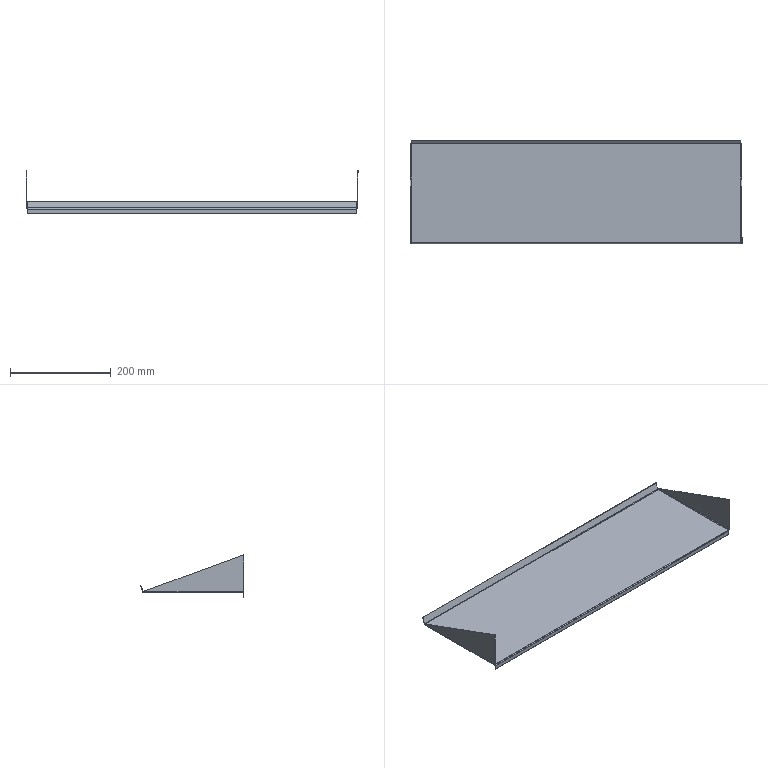Part | SolidWorks | features BaseBody 1 | 1 solid | 34 faces | box 660 x 205.13 x 84 mm | volume 161412 mm3 | plane 26 | cylinder 8 | commonest cylinder face diameters 2 x4 4 x4
STEP:
#1=CARTESIAN_POINT('',(-2.,2.,0.));
#2=VERTEX_POINT('',#1);
#3=CARTESIAN_POINT('',(-2.,198.6,0.));
#4=VERTEX_POINT('',#3);
#5=CARTESIAN_POINT('',(-2.,198.6,0.));
#6=DIRECTION('',(0.,1.,0.));
#7=VECTOR('',#6,1000.);
#8=LINE('',#5,#7);
#9=EDGE_CURVE('',#2,#4,#8,.T.);
#10=ORIENTED_EDGE('',*,*,#9,.F.);
#11=CARTESIAN_POINT('',(-658.,2.,0.));
#12=VERTEX_POINT('',#11);
#13=CARTESIAN_POINT('',(-660.262,2.,0.));
#14=DIRECTION('',(1.,0.,0.));
#15=VECTOR('',#14,1000.);
#16=LINE('',#13,#15);
#17=EDGE_CURVE('',#12,#2,#16,.T.);
#18=ORIENTED_EDGE('',*,*,#17,.F.);
#19=CARTESIAN_POINT('',(-658.,198.6,0.));
#20=VERTEX_POINT('',#19);
#21=CARTESIAN_POINT('',(-658.,198.6,0.));
#22=DIRECTION('',(0.,-1.,0.));
#23=VECTOR('',#22,1000.);
#24=LINE('',#21,#23);
#25=EDGE_CURVE('',#20,#12,#24,.T.);
#26=ORIENTED_EDGE('',*,*,#25,.F.);
#27=CARTESIAN_POINT('',(-660.262,198.6,0.));
#28=DIRECTION('',(-1.,0.,0.));
#29=VECTOR('',#28,1000.);
#30=LINE('',#27,#29);
#31=EDGE_CURVE('',#4,#20,#30,.T.);
#32=ORIENTED_EDGE('',*,*,#31,.F.);
#33=EDGE_LOOP('',(#10,#18,#26,#32));
#34=FACE_OUTER_BOUND('',#33,.T.);
#35=CARTESIAN_POINT('',(-660.262,198.6,0.));
#36=DIRECTION('',(0.,0.,1.));
#37=DIRECTION('',(1.,0.,0.));
#38=AXIS2_PLACEMENT_3D('',#35,#36,#37);
#39=PLANE('',#38);
#40=ADVANCED_FACE('',(#34),#39,.F.);
#41=CARTESIAN_POINT('',(-658.,200.479,1.316));
#42=VERTEX_POINT('',#41);
#43=CARTESIAN_POINT('',(-658.,198.6,2.));
#44=DIRECTION('',(1.,0.,0.));
#45=DIRECTION('',(0.,1.,0.));
#46=AXIS2_PLACEMENT_3D('',#43,#44,#45);
#47=CIRCLE('',#46,2.);
#48=EDGE_CURVE('',#20,#42,#47,.T.);
#49=ORIENTED_EDGE('',*,*,#48,.T.);
#50=CARTESIAN_POINT('',(-2.,200.479,1.316));
#51=VERTEX_POINT('',#50);
#52=CARTESIAN_POINT('',(-330.,200.479,1.316));
#53=DIRECTION('',(1.,0.,0.));
#54=VECTOR('',#53,1000.);
#55=LINE('',#52,#54);
#56=EDGE_CURVE('',#42,#51,#55,.T.);
#57=ORIENTED_EDGE('',*,*,#56,.T.);
#58=CARTESIAN_POINT('',(-2.,198.6,2.));
#59=DIRECTION('',(-1.,0.,0.));
#60=DIRECTION('',(0.,1.,0.));
#61=AXIS2_PLACEMENT_3D('',#58,#59,#60);
#62=CIRCLE('',#61,2.);
#63=EDGE_CURVE('',#51,#4,#62,.T.);
#64=ORIENTED_EDGE('',*,*,#63,.T.);
#65=ORIENTED_EDGE('',*,*,#31,.T.);
#66=EDGE_LOOP('',(#49,#57,#64,#65));
#67=FACE_OUTER_BOUND('',#66,.T.);
#68=CARTESIAN_POINT('',(-330.,198.6,2.));
#69=DIRECTION('',(1.,0.,0.));
#70=DIRECTION('',(0.,1.,0.));
#71=AXIS2_PLACEMENT_3D('',#68,#69,#70);
#72=CYLINDRICAL_SURFACE('',#71,2.);
#73=ADVANCED_FACE('',(#67),#72,.T.);
#74=CARTESIAN_POINT('',(0.,2.,2.));
#75=VERTEX_POINT('',#74);
#76=CARTESIAN_POINT('',(-2.,2.,2.));
#77=DIRECTION('',(0.,1.,0.));
#78=DIRECTION('',(1.,0.,0.));
#79=AXIS2_PLACEMENT_3D('',#76,#77,#78);
#80=CIRCLE('',#79,2.);
#81=EDGE_CURVE('',#75,#2,#80,.T.);
#82=ORIENTED_EDGE('',*,*,#81,.T.);
#83=ORIENTED_EDGE('',*,*,#9,.T.);
#84=CARTESIAN_POINT('',(0.,198.6,2.));
#85=VERTEX_POINT('',#84);
#86=CARTESIAN_POINT('',(-2.,198.6,2.));
#87=DIRECTION('',(0.,-1.,0.));
#88=DIRECTION('',(1.,0.,0.));
#89=AXIS2_PLACEMENT_3D('',#86,#87,#88);
#90=CIRCLE('',#89,2.);
#91=EDGE_CURVE('',#4,#85,#90,.T.);
#92=ORIENTED_EDGE('',*,*,#91,.T.);
#93=CARTESIAN_POINT('',(0.,100.,2.));
#94=DIRECTION('',(0.,-1.,0.));
#95=VECTOR('',#94,1000.);
#96=LINE('',#93,#95);
#97=EDGE_CURVE('',#85,#75,#96,.T.);
#98=ORIENTED_EDGE('',*,*,#97,.T.);
#99=EDGE_LOOP('',(#82,#83,#92,#98));
#100=FACE_OUTER_BOUND('',#99,.T.);
#101=CARTESIAN_POINT('',(-2.,100.,2.));
#102=DIRECTION('',(0.,-1.,0.));
#103=DIRECTION('',(1.,0.,0.));
#104=AXIS2_PLACEMENT_3D('',#101,#102,#103);
#105=CYLINDRICAL_SURFACE('',#104,2.);
#106=ADVANCED_FACE('',(#100),#105,.T.);
#107=CARTESIAN_POINT('',(-658.,1.,-1.));
#108=VERTEX_POINT('',#107);
#109=CARTESIAN_POINT('',(-658.,2.,-1.));
#110=DIRECTION('',(1.,0.,0.));
#111=DIRECTION('',(0.,1.,0.));
#112=AXIS2_PLACEMENT_3D('',#109,#110,#111);
#113=CIRCLE('',#112,1.);
#114=EDGE_CURVE('',#12,#108,#113,.T.);
#115=ORIENTED_EDGE('',*,*,#114,.F.);
#116=ORIENTED_EDGE('',*,*,#17,.T.);
#117=CARTESIAN_POINT('',(-2.,1.,-1.));
#118=VERTEX_POINT('',#117);
#119=CARTESIAN_POINT('',(-2.,2.,-1.));
#120=DIRECTION('',(-1.,0.,0.));
#121=DIRECTION('',(0.,1.,0.));
#122=AXIS2_PLACEMENT_3D('',#119,#120,#121);
#123=CIRCLE('',#122,1.);
#124=EDGE_CURVE('',#118,#2,#123,.T.);
#125=ORIENTED_EDGE('',*,*,#124,.F.);
#126=CARTESIAN_POINT('',(-330.,1.,-1.));
#127=DIRECTION('',(1.,0.,0.));
#128=VECTOR('',#127,1000.);
#129=LINE('',#126,#128);
#130=EDGE_CURVE('',#108,#118,#129,.T.);
#131=ORIENTED_EDGE('',*,*,#130,.F.);
#132=EDGE_LOOP('',(#115,#116,#125,#131));
#133=FACE_OUTER_BOUND('',#132,.T.);
#134=CARTESIAN_POINT('',(-330.,2.,-1.));
#135=DIRECTION('',(1.,0.,0.));
#136=DIRECTION('',(0.,1.,0.));
#137=AXIS2_PLACEMENT_3D('',#134,#135,#136);
#138=CYLINDRICAL_SURFACE('',#137,1.);
#139=ADVANCED_FACE('',(#133),#138,.F.);
#140=CARTESIAN_POINT('',(-660.,2.,2.));
#141=VERTEX_POINT('',#140);
#142=CARTESIAN_POINT('',(-658.,2.,2.));
#143=DIRECTION('',(0.,1.,0.));
#144=DIRECTION('',(0.,0.,1.));
#145=AXIS2_PLACEMENT_3D('',#142,#143,#144);
#146=CIRCLE('',#145,2.);
#147=EDGE_CURVE('',#12,#141,#146,.T.);
#148=ORIENTED_EDGE('',*,*,#147,.T.);
#149=CARTESIAN_POINT('',(-660.,198.6,2.));
#150=VERTEX_POINT('',#149);
#151=CARTESIAN_POINT('',(-660.,100.,2.));
#152=DIRECTION('',(0.,1.,0.));
#153=VECTOR('',#152,1000.);
#154=LINE('',#151,#153);
#155=EDGE_CURVE('',#141,#150,#154,.T.);
#156=ORIENTED_EDGE('',*,*,#155,.T.);
#157=CARTESIAN_POINT('',(-658.,198.6,2.));
#158=DIRECTION('',(0.,-1.,0.));
#159=DIRECTION('',(0.,0.,1.));
#160=AXIS2_PLACEMENT_3D('',#157,#158,#159);
#161=CIRCLE('',#160,2.);
#162=EDGE_CURVE('',#150,#20,#161,.T.);
#163=ORIENTED_EDGE('',*,*,#162,.T.);
#164=ORIENTED_EDGE('',*,*,#25,.T.);
#165=EDGE_LOOP('',(#148,#156,#163,#164));
#166=FACE_OUTER_BOUND('',#165,.T.);
#167=CARTESIAN_POINT('',(-658.,100.,2.));
#168=DIRECTION('',(0.,1.,0.));
#169=DIRECTION('',(0.,0.,1.));
#170=AXIS2_PLACEMENT_3D('',#167,#168,#169);
#171=CYLINDRICAL_SURFACE('',#170,2.);
#172=ADVANCED_FACE('',(#166),#171,.T.);
#173=ORIENTED_EDGE('',*,*,#48,.F.);
#174=CARTESIAN_POINT('',(-658.,198.6,1.));
#175=VERTEX_POINT('',#174);
#176=CARTESIAN_POINT('',(-658.,198.6,1.316));
#177=DIRECTION('',(0.,0.,1.));
#178=VECTOR('',#177,1000.);
#179=LINE('',#176,#178);
#180=EDGE_CURVE('',#20,#175,#179,.T.);
#181=ORIENTED_EDGE('',*,*,#180,.T.);
#182=CARTESIAN_POINT('',(-658.,199.539,1.658));
#183=VERTEX_POINT('',#182);
#184=CARTESIAN_POINT('',(-658.,198.6,2.));
#185=DIRECTION('',(1.,0.,0.));
#186=DIRECTION('',(0.,1.,0.));
#187=AXIS2_PLACEMENT_3D('',#184,#185,#186);
#188=CIRCLE('',#187,1.);
#189=EDGE_CURVE('',#175,#183,#188,.T.);
#190=ORIENTED_EDGE('',*,*,#189,.T.);
#191=CARTESIAN_POINT('',(-658.,204.191,14.437));
#192=VERTEX_POINT('',#191);
#193=CARTESIAN_POINT('',(-658.,199.539,1.658));
#194=DIRECTION('',(0.,0.342,0.9397));
#195=VECTOR('',#194,1000.);
#196=LINE('',#193,#195);
#197=EDGE_CURVE('',#183,#192,#196,.T.);
#198=ORIENTED_EDGE('',*,*,#197,.T.);
#199=CARTESIAN_POINT('',(-658.,205.13,14.095));
#200=VERTEX_POINT('',#199);
#201=CARTESIAN_POINT('',(-658.,204.191,14.437));
#202=DIRECTION('',(0.,0.9397,-0.342));
#203=VECTOR('',#202,1000.);
#204=LINE('',#201,#203);
#205=EDGE_CURVE('',#192,#200,#204,.T.);
#206=ORIENTED_EDGE('',*,*,#205,.T.);
#207=CARTESIAN_POINT('',(-658.,202.504,6.879));
#208=DIRECTION('',(0.,-0.342,-0.9397));
#209=VECTOR('',#208,1000.);
#210=LINE('',#207,#209);
#211=EDGE_CURVE('',#200,#42,#210,.T.);
#212=ORIENTED_EDGE('',*,*,#211,.T.);
#213=EDGE_LOOP('',(#173,#181,#190,#198,#206,#212));
#214=FACE_OUTER_BOUND('',#213,.T.);
#215=CARTESIAN_POINT('',(-658.,200.479,1.316));
#216=DIRECTION('',(-1.,0.,0.));
#217=DIRECTION('',(0.,-1.,0.));
#218=AXIS2_PLACEMENT_3D('',#215,#216,#217);
#219=PLANE('',#218);
#220=ADVANCED_FACE('',(#214),#219,.T.);
#221=CARTESIAN_POINT('',(-2.,198.6,1.));
#222=VERTEX_POINT('',#221);
#223=CARTESIAN_POINT('',(-2.,198.6,1.658));
#224=DIRECTION('',(0.,0.,-1.));
#225=VECTOR('',#224,1000.);
#226=LINE('',#223,#225);
#227=EDGE_CURVE('',#222,#4,#226,.T.);
#228=ORIENTED_EDGE('',*,*,#227,.T.);
#229=ORIENTED_EDGE('',*,*,#63,.F.);
#230=CARTESIAN_POINT('',(-2.,205.13,14.095));
#231=VERTEX_POINT('',#230);
#232=CARTESIAN_POINT('',(-2.,202.504,6.879));
#233=DIRECTION('',(0.,0.342,0.9397));
#234=VECTOR('',#233,1000.);
#235=LINE('',#232,#234);
#236=EDGE_CURVE('',#51,#231,#235,.T.);
#237=ORIENTED_EDGE('',*,*,#236,.T.);
#238=CARTESIAN_POINT('',(-2.,204.191,14.437));
#239=VERTEX_POINT('',#238);
#240=CARTESIAN_POINT('',(-2.,204.191,14.437));
#241=DIRECTION('',(0.,0.9397,-0.342));
#242=VECTOR('',#241,1000.);
#243=LINE('',#240,#242);
#244=EDGE_CURVE('',#239,#231,#243,.T.);
#245=ORIENTED_EDGE('',*,*,#244,.F.);
#246=CARTESIAN_POINT('',(-2.,199.539,1.658));
#247=VERTEX_POINT('',#246);
#248=CARTESIAN_POINT('',(-2.,204.191,14.437));
#249=DIRECTION('',(0.,-0.342,-0.9397));
#250=VECTOR('',#249,1000.);
#251=LINE('',#248,#250);
#252=EDGE_CURVE('',#239,#247,#251,.T.);
#253=ORIENTED_EDGE('',*,*,#252,.T.);
#254=CARTESIAN_POINT('',(-2.,198.6,2.));
#255=DIRECTION('',(-1.,0.,0.));
#256=DIRECTION('',(0.,1.,0.));
#257=AXIS2_PLACEMENT_3D('',#254,#255,#256);
#258=CIRCLE('',#257,1.);
#259=EDGE_CURVE('',#247,#222,#258,.T.);
#260=ORIENTED_EDGE('',*,*,#259,.T.);
#261=EDGE_LOOP('',(#228,#229,#237,#245,#253,#260));
#262=FACE_OUTER_BOUND('',#261,.T.);
#263=CARTESIAN_POINT('',(-2.,199.539,1.658));
#264=DIRECTION('',(1.,0.,0.));
#265=DIRECTION('',(0.,1.,0.));
#266=AXIS2_PLACEMENT_3D('',#263,#264,#265);
#267=PLANE('',#266);
#268=ADVANCED_FACE('',(#262),#267,.T.);
#269=ORIENTED_EDGE('',*,*,#211,.F.);
#270=CARTESIAN_POINT('',(-330.,205.13,14.095));
#271=DIRECTION('',(-1.,0.,0.));
#272=VECTOR('',#271,1000.);
#273=LINE('',#270,#272);
#274=EDGE_CURVE('',#231,#200,#273,.T.);
#275=ORIENTED_EDGE('',*,*,#274,.F.);
#276=ORIENTED_EDGE('',*,*,#236,.F.);
#277=ORIENTED_EDGE('',*,*,#56,.F.);
#278=EDGE_LOOP('',(#269,#275,#276,#277));
#279=FACE_OUTER_BOUND('',#278,.T.);
#280=CARTESIAN_POINT('',(-330.,202.504,6.879));
#281=DIRECTION('',(0.,-0.9397,0.342));
#282=DIRECTION('',(0.,-0.342,-0.9397));
#283=AXIS2_PLACEMENT_3D('',#280,#281,#282);
#284=PLANE('',#283);
#285=ADVANCED_FACE('',(#279),#284,.F.);
#286=CARTESIAN_POINT('',(-1.,2.,2.));
#287=VERTEX_POINT('',#286);
#288=CARTESIAN_POINT('',(-1.,2.,2.));
#289=DIRECTION('',(-1.,0.,0.));
#290=VECTOR('',#289,1000.);
#291=LINE('',#288,#290);
#292=EDGE_CURVE('',#75,#287,#291,.T.);
#293=ORIENTED_EDGE('',*,*,#292,.T.);
#294=CARTESIAN_POINT('',(-2.,2.,1.));
#295=VERTEX_POINT('',#294);
#296=CARTESIAN_POINT('',(-2.,2.,2.));
#297=DIRECTION('',(0.,1.,0.));
#298=DIRECTION('',(1.,0.,0.));
#299=AXIS2_PLACEMENT_3D('',#296,#297,#298);
#300=CIRCLE('',#299,1.);
#301=EDGE_CURVE('',#287,#295,#300,.T.);
#302=ORIENTED_EDGE('',*,*,#301,.T.);
#303=CARTESIAN_POINT('',(-2.,2.,-1.));
#304=DIRECTION('',(0.,0.,1.));
#305=VECTOR('',#304,1000.);
#306=LINE('',#303,#305);
#307=EDGE_CURVE('',#2,#295,#306,.T.);
#308=ORIENTED_EDGE('',*,*,#307,.F.);
#309=ORIENTED_EDGE('',*,*,#81,.F.);
#310=EDGE_LOOP('',(#293,#302,#308,#309));
#311=FACE_OUTER_BOUND('',#310,.T.);
#312=CARTESIAN_POINT('',(0.,2.,2.));
#313=DIRECTION('',(0.,1.,0.));
#314=DIRECTION('',(-1.,0.,0.));
#315=AXIS2_PLACEMENT_3D('',#312,#313,#314);
#316=PLANE('',#315);
#317=ADVANCED_FACE('',(#311),#316,.F.);
#318=CARTESIAN_POINT('',(0.,0.,75.));
#319=VERTEX_POINT('',#318);
#320=CARTESIAN_POINT('',(0.,198.6,2.511));
#321=VERTEX_POINT('',#320);
#322=CARTESIAN_POINT('',(0.,0.,75.));
#323=DIRECTION('',(0.,0.9394,-0.3429));
#324=VECTOR('',#323,1000.);
#325=LINE('',#322,#324);
#326=EDGE_CURVE('',#319,#321,#325,.T.);
#327=ORIENTED_EDGE('',*,*,#326,.F.);
#328=CARTESIAN_POINT('',(0.,0.,2.));
#329=VERTEX_POINT('',#328);
#330=CARTESIAN_POINT('',(0.,0.,-658.524));
#331=DIRECTION('',(0.,0.,1.));
#332=VECTOR('',#331,1000.);
#333=LINE('',#330,#332);
#334=EDGE_CURVE('',#329,#319,#333,.T.);
#335=ORIENTED_EDGE('',*,*,#334,.F.);
#336=CARTESIAN_POINT('',(0.,198.6,2.));
#337=DIRECTION('',(0.,-1.,0.));
#338=VECTOR('',#337,1000.);
#339=LINE('',#336,#338);
#340=EDGE_CURVE('',#75,#329,#339,.T.);
#341=ORIENTED_EDGE('',*,*,#340,.F.);
#342=ORIENTED_EDGE('',*,*,#97,.F.);
#343=CARTESIAN_POINT('',(0.,198.6,-658.524));
#344=DIRECTION('',(0.,0.,-1.));
#345=VECTOR('',#344,1000.);
#346=LINE('',#343,#345);
#347=EDGE_CURVE('',#321,#85,#346,.T.);
#348=ORIENTED_EDGE('',*,*,#347,.F.);
#349=EDGE_LOOP('',(#327,#335,#341,#342,#348));
#350=FACE_OUTER_BOUND('',#349,.T.);
#351=CARTESIAN_POINT('',(0.,198.6,-658.524));
#352=DIRECTION('',(-1.,0.,0.));
#353=DIRECTION('',(0.,0.,1.));
#354=AXIS2_PLACEMENT_3D('',#351,#352,#353);
#355=PLANE('',#354);
#356=ADVANCED_FACE('',(#350),#355,.F.);
#357=ORIENTED_EDGE('',*,*,#91,.F.);
#358=ORIENTED_EDGE('',*,*,#227,.F.);
#359=CARTESIAN_POINT('',(-1.,198.6,2.));
#360=VERTEX_POINT('',#359);
#361=CARTESIAN_POINT('',(-2.,198.6,2.));
#362=DIRECTION('',(0.,-1.,0.));
#363=DIRECTION('',(1.,0.,0.));
#364=AXIS2_PLACEMENT_3D('',#361,#362,#363);
#365=CIRCLE('',#364,1.);
#366=EDGE_CURVE('',#222,#360,#365,.T.);
#367=ORIENTED_EDGE('',*,*,#366,.T.);
#368=CARTESIAN_POINT('',(-1.,198.6,2.511));
#369=VERTEX_POINT('',#368);
#370=CARTESIAN_POINT('',(-1.,198.6,-328.262));
#371=DIRECTION('',(0.,0.,-1.));
#372=VECTOR('',#371,1000.);
#373=LINE('',#370,#372);
#374=EDGE_CURVE('',#369,#360,#373,.T.);
#375=ORIENTED_EDGE('',*,*,#374,.F.);
#376=CARTESIAN_POINT('',(-1.,198.6,2.511));
#377=DIRECTION('',(-1.,0.,0.));
#378=VECTOR('',#377,1000.);
#379=LINE('',#376,#378);
#380=EDGE_CURVE('',#321,#369,#379,.T.);
#381=ORIENTED_EDGE('',*,*,#380,.F.);
#382=ORIENTED_EDGE('',*,*,#347,.T.);
#383=EDGE_LOOP('',(#357,#358,#367,#375,#381,#382));
#384=FACE_OUTER_BOUND('',#383,.T.);
#385=CARTESIAN_POINT('',(-1.,198.6,2.));
#386=DIRECTION('',(0.,1.,0.));
#387=DIRECTION('',(-1.,0.,0.));
#388=AXIS2_PLACEMENT_3D('',#385,#386,#387);
#389=PLANE('',#388);
#390=ADVANCED_FACE('',(#384),#389,.T.);
#391=CARTESIAN_POINT('',(-2.,1.,-9.));
#392=VERTEX_POINT('',#391);
#393=CARTESIAN_POINT('',(-2.,1.,-3.869));
#394=DIRECTION('',(0.,0.,1.));
#395=VECTOR('',#394,1000.);
#396=LINE('',#393,#395);
#397=EDGE_CURVE('',#392,#118,#396,.T.);
#398=ORIENTED_EDGE('',*,*,#397,.F.);
#399=CARTESIAN_POINT('',(-658.,1.,-9.));
#400=VERTEX_POINT('',#399);
#401=CARTESIAN_POINT('',(-330.,1.,-9.));
#402=DIRECTION('',(1.,0.,0.));
#403=VECTOR('',#402,1000.);
#404=LINE('',#401,#403);
#405=EDGE_CURVE('',#400,#392,#404,.T.);
#406=ORIENTED_EDGE('',*,*,#405,.F.);
#407=CARTESIAN_POINT('',(-658.,1.,-3.869));
#408=DIRECTION('',(0.,0.,-1.));
#409=VECTOR('',#408,1000.);
#410=LINE('',#407,#409);
#411=EDGE_CURVE('',#108,#400,#410,.T.);
#412=ORIENTED_EDGE('',*,*,#411,.F.);
#413=ORIENTED_EDGE('',*,*,#130,.T.);
#414=EDGE_LOOP('',(#398,#406,#412,#413));
#415=FACE_OUTER_BOUND('',#414,.T.);
#416=CARTESIAN_POINT('',(-330.,1.,-3.869));
#417=DIRECTION('',(0.,-1.,0.));
#418=DIRECTION('',(1.,0.,0.));
#419=AXIS2_PLACEMENT_3D('',#416,#417,#418);
#420=PLANE('',#419);
#421=ADVANCED_FACE('',(#415),#420,.F.);
#422=ORIENTED_EDGE('',*,*,#155,.F.);
#423=CARTESIAN_POINT('',(-660.,0.,2.));
#424=VERTEX_POINT('',#423);
#425=CARTESIAN_POINT('',(-660.,198.6,2.));
#426=DIRECTION('',(0.,1.,0.));
#427=VECTOR('',#426,1000.);
#428=LINE('',#425,#427);
#429=EDGE_CURVE('',#424,#141,#428,.T.);
#430=ORIENTED_EDGE('',*,*,#429,.F.);
#431=CARTESIAN_POINT('',(-660.,0.,75.));
#432=VERTEX_POINT('',#431);
#433=CARTESIAN_POINT('',(-660.,0.,2.));
#434=DIRECTION('',(0.,0.,-1.));
#435=VECTOR('',#434,1000.);
#436=LINE('',#433,#435);
#437=EDGE_CURVE('',#432,#424,#436,.T.);
#438=ORIENTED_EDGE('',*,*,#437,.F.);
#439=CARTESIAN_POINT('',(-660.,198.6,2.511));
#440=VERTEX_POINT('',#439);
#441=CARTESIAN_POINT('',(-660.,198.6,2.511));
#442=DIRECTION('',(0.,-0.9394,0.3429));
#443=VECTOR('',#442,1000.);
#444=LINE('',#441,#443);
#445=EDGE_CURVE('',#440,#432,#444,.T.);
#446=ORIENTED_EDGE('',*,*,#445,.F.);
#447=CARTESIAN_POINT('',(-660.,198.6,2.));
#448=DIRECTION('',(0.,0.,1.));
#449=VECTOR('',#448,1000.);
#450=LINE('',#447,#449);
#451=EDGE_CURVE('',#150,#440,#450,.T.);
#452=ORIENTED_EDGE('',*,*,#451,.F.);
#453=EDGE_LOOP('',(#422,#430,#438,#446,#452));
#454=FACE_OUTER_BOUND('',#453,.T.);
#455=CARTESIAN_POINT('',(-660.,198.6,2.));
#456=DIRECTION('',(1.,0.,0.));
#457=DIRECTION('',(0.,0.,-1.));
#458=AXIS2_PLACEMENT_3D('',#455,#456,#457);
#459=PLANE('',#458);
#460=ADVANCED_FACE('',(#454),#459,.F.);
#461=CARTESIAN_POINT('',(-658.,2.,1.));
#462=VERTEX_POINT('',#461);
#463=CARTESIAN_POINT('',(-658.,2.,-1.));
#464=DIRECTION('',(0.,0.,-1.));
#465=VECTOR('',#464,1000.);
#466=LINE('',#463,#465);
#467=EDGE_CURVE('',#462,#12,#466,.T.);
#468=ORIENTED_EDGE('',*,*,#467,.F.);
#469=CARTESIAN_POINT('',(-659.,2.,2.));
#470=VERTEX_POINT('',#469);
#471=CARTESIAN_POINT('',(-658.,2.,2.));
#472=DIRECTION('',(0.,1.,0.));
#473=DIRECTION('',(0.,0.,1.));
#474=AXIS2_PLACEMENT_3D('',#471,#472,#473);
#475=CIRCLE('',#474,1.);
#476=EDGE_CURVE('',#462,#470,#475,.T.);
#477=ORIENTED_EDGE('',*,*,#476,.T.);
#478=CARTESIAN_POINT('',(-658.,2.,2.));
#479=DIRECTION('',(1.,0.,0.));
#480=VECTOR('',#479,1000.);
#481=LINE('',#478,#480);
#482=EDGE_CURVE('',#141,#470,#481,.T.);
#483=ORIENTED_EDGE('',*,*,#482,.F.);
#484=ORIENTED_EDGE('',*,*,#147,.F.);
#485=EDGE_LOOP('',(#468,#477,#483,#484));
#486=FACE_OUTER_BOUND('',#485,.T.);
#487=CARTESIAN_POINT('',(-658.,2.,0.));
#488=DIRECTION('',(0.,1.,0.));
#489=DIRECTION('',(0.,0.,1.));
#490=AXIS2_PLACEMENT_3D('',#487,#488,#489);
#491=PLANE('',#490);
#492=ADVANCED_FACE('',(#486),#491,.F.);
#493=ORIENTED_EDGE('',*,*,#162,.F.);
#494=ORIENTED_EDGE('',*,*,#451,.T.);
#495=CARTESIAN_POINT('',(-659.,198.6,2.511));
#496=VERTEX_POINT('',#495);
#497=CARTESIAN_POINT('',(-659.,198.6,2.511));
#498=DIRECTION('',(-1.,0.,0.));
#499=VECTOR('',#498,1000.);
#500=LINE('',#497,#499);
#501=EDGE_CURVE('',#496,#440,#500,.T.);
#502=ORIENTED_EDGE('',*,*,#501,.F.);
#503=CARTESIAN_POINT('',(-659.,198.6,2.));
#504=VERTEX_POINT('',#503);
#505=CARTESIAN_POINT('',(-659.,198.6,-328.262));
#506=DIRECTION('',(0.,0.,1.));
#507=VECTOR('',#506,1000.);
#508=LINE('',#505,#507);
#509=EDGE_CURVE('',#504,#496,#508,.T.);
#510=ORIENTED_EDGE('',*,*,#509,.F.);
#511=CARTESIAN_POINT('',(-658.,198.6,2.));
#512=DIRECTION('',(0.,-1.,0.));
#513=DIRECTION('',(0.,0.,1.));
#514=AXIS2_PLACEMENT_3D('',#511,#512,#513);
#515=CIRCLE('',#514,1.);
#516=EDGE_CURVE('',#504,#175,#515,.T.);
#517=ORIENTED_EDGE('',*,*,#516,.T.);
#518=ORIENTED_EDGE('',*,*,#180,.F.);
#519=EDGE_LOOP('',(#493,#494,#502,#510,#517,#518));
#520=FACE_OUTER_BOUND('',#519,.T.);
#521=CARTESIAN_POINT('',(-658.,198.6,1.));
#522=DIRECTION('',(0.,1.,0.));
#523=DIRECTION('',(0.,0.,1.));
#524=AXIS2_PLACEMENT_3D('',#521,#522,#523);
#525=PLANE('',#524);
#526=ADVANCED_FACE('',(#520),#525,.T.);
#527=CARTESIAN_POINT('',(-2.,204.191,14.437));
#528=DIRECTION('',(1.,0.,0.));
#529=VECTOR('',#528,1000.);
#530=LINE('',#527,#529);
#531=EDGE_CURVE('',#192,#239,#530,.T.);
#532=ORIENTED_EDGE('',*,*,#531,.T.);
#533=ORIENTED_EDGE('',*,*,#244,.T.);
#534=ORIENTED_EDGE('',*,*,#274,.T.);
#535=ORIENTED_EDGE('',*,*,#205,.F.);
#536=EDGE_LOOP('',(#532,#533,#534,#535));
#537=FACE_OUTER_BOUND('',#536,.T.);
#538=CARTESIAN_POINT('',(-2.,204.191,14.437));
#539=DIRECTION('',(0.,0.342,0.9397));
#540=DIRECTION('',(0.,-0.9397,0.342));
#541=AXIS2_PLACEMENT_3D('',#538,#539,#540);
#542=PLANE('',#541);
#543=ADVANCED_FACE('',(#537),#542,.T.);
#544=CARTESIAN_POINT('',(-1.,0.,75.));
#545=VERTEX_POINT('',#544);
#546=CARTESIAN_POINT('',(-1.,0.,75.));
#547=DIRECTION('',(0.,0.9394,-0.3429));
#548=VECTOR('',#547,1000.);
#549=LINE('',#546,#548);
#550=EDGE_CURVE('',#545,#369,#549,.T.);
#551=ORIENTED_EDGE('',*,*,#550,.F.);
#552=CARTESIAN_POINT('',(-660.,0.,75.));
#553=DIRECTION('',(-1.,0.,0.));
#554=VECTOR('',#553,1000.);
#555=LINE('',#552,#554);
#556=EDGE_CURVE('',#319,#545,#555,.T.);
#557=ORIENTED_EDGE('',*,*,#556,.F.);
#558=ORIENTED_EDGE('',*,*,#326,.T.);
#559=ORIENTED_EDGE('',*,*,#380,.T.);
#560=EDGE_LOOP('',(#551,#557,#558,#559));
#561=FACE_OUTER_BOUND('',#560,.T.);
#562=CARTESIAN_POINT('',(-660.,0.,75.));
#563=DIRECTION('',(0.,-0.3429,-0.9394));
#564=DIRECTION('',(0.,0.9394,-0.3429));
#565=AXIS2_PLACEMENT_3D('',#562,#563,#564);
#566=PLANE('',#565);
#567=ADVANCED_FACE('',(#561),#566,.F.);
#568=ORIENTED_EDGE('',*,*,#556,.T.);
#569=CARTESIAN_POINT('',(-1.,0.,2.));
#570=VERTEX_POINT('',#569);
#571=CARTESIAN_POINT('',(-1.,0.,2.));
#572=DIRECTION('',(0.,0.,-1.));
#573=VECTOR('',#572,1000.);
#574=LINE('',#571,#573);
#575=EDGE_CURVE('',#545,#570,#574,.T.);
#576=ORIENTED_EDGE('',*,*,#575,.T.);
#577=CARTESIAN_POINT('',(-1.,0.,2.));
#578=DIRECTION('',(1.,0.,0.));
#579=VECTOR('',#578,1000.);
#580=LINE('',#577,#579);
#581=EDGE_CURVE('',#570,#329,#580,.T.);
#582=ORIENTED_EDGE('',*,*,#581,.T.);
#583=ORIENTED_EDGE('',*,*,#334,.T.);
#584=EDGE_LOOP('',(#568,#576,#582,#583));
#585=FACE_OUTER_BOUND('',#584,.T.);
#586=CARTESIAN_POINT('',(-1.,0.,2.));
#587=DIRECTION('',(0.,-1.,0.));
#588=DIRECTION('',(1.,0.,0.));
#589=AXIS2_PLACEMENT_3D('',#586,#587,#588);
#590=PLANE('',#589);
#591=ADVANCED_FACE('',(#585),#590,.T.);
#592=CARTESIAN_POINT('',(-1.,2.,2.));
#593=DIRECTION('',(0.,-1.,0.));
#594=VECTOR('',#593,1000.);
#595=LINE('',#592,#594);
#596=EDGE_CURVE('',#287,#570,#595,.T.);
#597=ORIENTED_EDGE('',*,*,#596,.F.);
#598=ORIENTED_EDGE('',*,*,#292,.F.);
#599=ORIENTED_EDGE('',*,*,#340,.T.);
#600=ORIENTED_EDGE('',*,*,#581,.F.);
#601=EDGE_LOOP('',(#597,#598,#599,#600));
#602=FACE_OUTER_BOUND('',#601,.T.);
#603=CARTESIAN_POINT('',(-1.,2.,2.));
#604=DIRECTION('',(0.,0.,1.));
#605=DIRECTION('',(1.,0.,0.));
#606=AXIS2_PLACEMENT_3D('',#603,#604,#605);
#607=PLANE('',#606);
#608=ADVANCED_FACE('',(#602),#607,.F.);
#609=CARTESIAN_POINT('',(-2.,0.,-9.));
#610=VERTEX_POINT('',#609);
#611=CARTESIAN_POINT('',(-2.,1.,-9.));
#612=DIRECTION('',(0.,1.,0.));
#613=VECTOR('',#612,1000.);
#614=LINE('',#611,#613);
#615=EDGE_CURVE('',#610,#392,#614,.T.);
#616=ORIENTED_EDGE('',*,*,#615,.T.);
#617=ORIENTED_EDGE('',*,*,#397,.T.);
#618=ORIENTED_EDGE('',*,*,#124,.T.);
#619=ORIENTED_EDGE('',*,*,#307,.T.);
#620=CARTESIAN_POINT('',(-2.,0.,-1.));
#621=VERTEX_POINT('',#620);
#622=CARTESIAN_POINT('',(-2.,2.,-1.));
#623=DIRECTION('',(-1.,0.,0.));
#624=DIRECTION('',(0.,1.,0.));
#625=AXIS2_PLACEMENT_3D('',#622,#623,#624);
#626=CIRCLE('',#625,2.);
#627=EDGE_CURVE('',#621,#295,#626,.T.);
#628=ORIENTED_EDGE('',*,*,#627,.F.);
#629=CARTESIAN_POINT('',(-2.,0.,-1.));
#630=DIRECTION('',(0.,0.,-1.));
#631=VECTOR('',#630,1000.);
#632=LINE('',#629,#631);
#633=EDGE_CURVE('',#621,#610,#632,.T.);
#634=ORIENTED_EDGE('',*,*,#633,.T.);
#635=EDGE_LOOP('',(#616,#617,#618,#619,#628,#634));
#636=FACE_OUTER_BOUND('',#635,.T.);
#637=CARTESIAN_POINT('',(-2.,1.,-1.));
#638=DIRECTION('',(1.,0.,0.));
#639=DIRECTION('',(0.,1.,0.));
#640=AXIS2_PLACEMENT_3D('',#637,#638,#639);
#641=PLANE('',#640);
#642=ADVANCED_FACE('',(#636),#641,.T.);
#643=ORIENTED_EDGE('',*,*,#405,.T.);
#644=ORIENTED_EDGE('',*,*,#615,.F.);
#645=CARTESIAN_POINT('',(-658.,0.,-9.));
#646=VERTEX_POINT('',#645);
#647=CARTESIAN_POINT('',(-2.,0.,-9.));
#648=DIRECTION('',(-1.,0.,0.));
#649=VECTOR('',#648,1000.);
#650=LINE('',#647,#649);
#651=EDGE_CURVE('',#610,#646,#650,.T.);
#652=ORIENTED_EDGE('',*,*,#651,.T.);
#653=CARTESIAN_POINT('',(-658.,1.,-9.));
#654=DIRECTION('',(0.,1.,0.));
#655=VECTOR('',#654,1000.);
#656=LINE('',#653,#655);
#657=EDGE_CURVE('',#646,#400,#656,.T.);
#658=ORIENTED_EDGE('',*,*,#657,.T.);
#659=EDGE_LOOP('',(#643,#644,#652,#658));
#660=FACE_OUTER_BOUND('',#659,.T.);
#661=CARTESIAN_POINT('',(-2.,1.,-9.));
#662=DIRECTION('',(0.,0.,-1.));
#663=DIRECTION('',(0.,1.,0.));
#664=AXIS2_PLACEMENT_3D('',#661,#662,#663);
#665=PLANE('',#664);
#666=ADVANCED_FACE('',(#660),#665,.T.);
#667=ORIENTED_EDGE('',*,*,#657,.F.);
#668=CARTESIAN_POINT('',(-658.,0.,-1.));
#669=VERTEX_POINT('',#668);
#670=CARTESIAN_POINT('',(-658.,0.,-1.));
#671=DIRECTION('',(0.,0.,1.));
#672=VECTOR('',#671,1000.);
#673=LINE('',#670,#672);
#674=EDGE_CURVE('',#646,#669,#673,.T.);
#675=ORIENTED_EDGE('',*,*,#674,.T.);
#676=CARTESIAN_POINT('',(-658.,2.,-1.));
#677=DIRECTION('',(1.,0.,0.));
#678=DIRECTION('',(0.,1.,0.));
#679=AXIS2_PLACEMENT_3D('',#676,#677,#678);
#680=CIRCLE('',#679,2.);
#681=EDGE_CURVE('',#462,#669,#680,.T.);
#682=ORIENTED_EDGE('',*,*,#681,.F.);
#683=ORIENTED_EDGE('',*,*,#467,.T.);
#684=ORIENTED_EDGE('',*,*,#114,.T.);
#685=ORIENTED_EDGE('',*,*,#411,.T.);
#686=EDGE_LOOP('',(#667,#675,#682,#683,#684,#685));
#687=FACE_OUTER_BOUND('',#686,.T.);
#688=CARTESIAN_POINT('',(-658.,1.,-1.));
#689=DIRECTION('',(-1.,0.,0.));
#690=DIRECTION('',(0.,-1.,0.));
#691=AXIS2_PLACEMENT_3D('',#688,#689,#690);
#692=PLANE('',#691);
#693=ADVANCED_FACE('',(#687),#692,.T.);
#694=ORIENTED_EDGE('',*,*,#429,.T.);
#695=ORIENTED_EDGE('',*,*,#482,.T.);
#696=CARTESIAN_POINT('',(-659.,0.,2.));
#697=VERTEX_POINT('',#696);
#698=CARTESIAN_POINT('',(-659.,2.,2.));
#699=DIRECTION('',(0.,1.,0.));
#700=VECTOR('',#699,1000.);
#701=LINE('',#698,#700);
#702=EDGE_CURVE('',#697,#470,#701,.T.);
#703=ORIENTED_EDGE('',*,*,#702,.F.);
#704=CARTESIAN_POINT('',(-660.,0.,2.));
#705=DIRECTION('',(1.,0.,0.));
#706=VECTOR('',#705,1000.);
#707=LINE('',#704,#706);
#708=EDGE_CURVE('',#424,#697,#707,.T.);
#709=ORIENTED_EDGE('',*,*,#708,.F.);
#710=EDGE_LOOP('',(#694,#695,#703,#709));
#711=FACE_OUTER_BOUND('',#710,.T.);
#712=CARTESIAN_POINT('',(-660.,2.,2.));
#713=DIRECTION('',(0.,0.,1.));
#714=DIRECTION('',(1.,0.,0.));
#715=AXIS2_PLACEMENT_3D('',#712,#713,#714);
#716=PLANE('',#715);
#717=ADVANCED_FACE('',(#711),#716,.F.);
#718=CARTESIAN_POINT('',(-659.,0.,75.));
#719=VERTEX_POINT('',#718);
#720=CARTESIAN_POINT('',(-659.,0.,75.));
#721=DIRECTION('',(-1.,0.,0.));
#722=VECTOR('',#721,1000.);
#723=LINE('',#720,#722);
#724=EDGE_CURVE('',#719,#432,#723,.T.);
#725=ORIENTED_EDGE('',*,*,#724,.T.);
#726=ORIENTED_EDGE('',*,*,#437,.T.);
#727=ORIENTED_EDGE('',*,*,#708,.T.);
#728=CARTESIAN_POINT('',(-659.,0.,2.));
#729=DIRECTION('',(0.,0.,1.));
#730=VECTOR('',#729,1000.);
#731=LINE('',#728,#730);
#732=EDGE_CURVE('',#697,#719,#731,.T.);
#733=ORIENTED_EDGE('',*,*,#732,.T.);
#734=EDGE_LOOP('',(#725,#726,#727,#733));
#735=FACE_OUTER_BOUND('',#734,.T.);
#736=CARTESIAN_POINT('',(-659.,0.,2.));
#737=DIRECTION('',(0.,-1.,0.));
#738=DIRECTION('',(0.,0.,-1.));
#739=AXIS2_PLACEMENT_3D('',#736,#737,#738);
#740=PLANE('',#739);
#741=ADVANCED_FACE('',(#735),#740,.T.);
#742=ORIENTED_EDGE('',*,*,#445,.T.);
#743=ORIENTED_EDGE('',*,*,#724,.F.);
#744=CARTESIAN_POINT('',(-659.,0.,75.));
#745=DIRECTION('',(0.,-0.9394,0.3429));
#746=VECTOR('',#745,1000.);
#747=LINE('',#744,#746);
#748=EDGE_CURVE('',#496,#719,#747,.T.);
#749=ORIENTED_EDGE('',*,*,#748,.F.);
#750=ORIENTED_EDGE('',*,*,#501,.T.);
#751=EDGE_LOOP('',(#742,#743,#749,#750));
#752=FACE_OUTER_BOUND('',#751,.T.);
#753=CARTESIAN_POINT('',(-660.,0.,75.));
#754=DIRECTION('',(0.,-0.3429,-0.9394));
#755=DIRECTION('',(0.,0.9394,-0.3429));
#756=AXIS2_PLACEMENT_3D('',#753,#754,#755);
#757=PLANE('',#756);
#758=ADVANCED_FACE('',(#752),#757,.F.);
#759=ORIENTED_EDGE('',*,*,#531,.F.);
#760=ORIENTED_EDGE('',*,*,#197,.F.);
#761=CARTESIAN_POINT('',(-330.,199.539,1.658));
#762=DIRECTION('',(1.,0.,0.));
#763=VECTOR('',#762,1000.);
#764=LINE('',#761,#763);
#765=EDGE_CURVE('',#183,#247,#764,.T.);
#766=ORIENTED_EDGE('',*,*,#765,.T.);
#767=ORIENTED_EDGE('',*,*,#252,.F.);
#768=EDGE_LOOP('',(#759,#760,#766,#767));
#769=FACE_OUTER_BOUND('',#768,.T.);
#770=CARTESIAN_POINT('',(-330.,201.564,7.221));
#771=DIRECTION('',(0.,-0.9397,0.342));
#772=DIRECTION('',(0.,-0.342,-0.9397));
#773=AXIS2_PLACEMENT_3D('',#770,#771,#772);
#774=PLANE('',#773);
#775=ADVANCED_FACE('',(#769),#774,.T.);
#776=ORIENTED_EDGE('',*,*,#575,.F.);
#777=ORIENTED_EDGE('',*,*,#550,.T.);
#778=ORIENTED_EDGE('',*,*,#374,.T.);
#779=CARTESIAN_POINT('',(-1.,100.,2.));
#780=DIRECTION('',(0.,-1.,0.));
#781=VECTOR('',#780,1000.);
#782=LINE('',#779,#781);
#783=EDGE_CURVE('',#360,#287,#782,.T.);
#784=ORIENTED_EDGE('',*,*,#783,.T.);
#785=ORIENTED_EDGE('',*,*,#596,.T.);
#786=EDGE_LOOP('',(#776,#777,#778,#784,#785));
#787=FACE_OUTER_BOUND('',#786,.T.);
#788=CARTESIAN_POINT('',(-1.,100.,-328.262));
#789=DIRECTION('',(-1.,0.,0.));
#790=DIRECTION('',(0.,0.,1.));
#791=AXIS2_PLACEMENT_3D('',#788,#789,#790);
#792=PLANE('',#791);
#793=ADVANCED_FACE('',(#787),#792,.T.);
#794=ORIENTED_EDGE('',*,*,#651,.F.);
#795=ORIENTED_EDGE('',*,*,#633,.F.);
#796=CARTESIAN_POINT('',(-330.,0.,-1.));
#797=DIRECTION('',(-1.,0.,0.));
#798=VECTOR('',#797,1000.);
#799=LINE('',#796,#798);
#800=EDGE_CURVE('',#621,#669,#799,.T.);
#801=ORIENTED_EDGE('',*,*,#800,.T.);
#802=ORIENTED_EDGE('',*,*,#674,.F.);
#803=EDGE_LOOP('',(#794,#795,#801,#802));
#804=FACE_OUTER_BOUND('',#803,.T.);
#805=CARTESIAN_POINT('',(-330.,0.,-3.869));
#806=DIRECTION('',(0.,-1.,0.));
#807=DIRECTION('',(1.,0.,0.));
#808=AXIS2_PLACEMENT_3D('',#805,#806,#807);
#809=PLANE('',#808);
#810=ADVANCED_FACE('',(#804),#809,.T.);
#811=ORIENTED_EDGE('',*,*,#702,.T.);
#812=CARTESIAN_POINT('',(-659.,100.,2.));
#813=DIRECTION('',(0.,1.,0.));
#814=VECTOR('',#813,1000.);
#815=LINE('',#812,#814);
#816=EDGE_CURVE('',#470,#504,#815,.T.);
#817=ORIENTED_EDGE('',*,*,#816,.T.);
#818=ORIENTED_EDGE('',*,*,#509,.T.);
#819=ORIENTED_EDGE('',*,*,#748,.T.);
#820=ORIENTED_EDGE('',*,*,#732,.F.);
#821=EDGE_LOOP('',(#811,#817,#818,#819,#820));
#822=FACE_OUTER_BOUND('',#821,.T.);
#823=CARTESIAN_POINT('',(-659.,100.,-328.262));
#824=DIRECTION('',(1.,0.,0.));
#825=DIRECTION('',(0.,0.,-1.));
#826=AXIS2_PLACEMENT_3D('',#823,#824,#825);
#827=PLANE('',#826);
#828=ADVANCED_FACE('',(#822),#827,.T.);
#829=ORIENTED_EDGE('',*,*,#189,.F.);
#830=CARTESIAN_POINT('',(-330.,198.6,1.));
#831=DIRECTION('',(-1.,0.,0.));
#832=VECTOR('',#831,1000.);
#833=LINE('',#830,#832);
#834=EDGE_CURVE('',#222,#175,#833,.T.);
#835=ORIENTED_EDGE('',*,*,#834,.F.);
#836=ORIENTED_EDGE('',*,*,#259,.F.);
#837=ORIENTED_EDGE('',*,*,#765,.F.);
#838=EDGE_LOOP('',(#829,#835,#836,#837));
#839=FACE_OUTER_BOUND('',#838,.T.);
#840=CARTESIAN_POINT('',(-330.,198.6,2.));
#841=DIRECTION('',(1.,0.,0.));
#842=DIRECTION('',(0.,1.,0.));
#843=AXIS2_PLACEMENT_3D('',#840,#841,#842);
#844=CYLINDRICAL_SURFACE('',#843,1.);
#845=ADVANCED_FACE('',(#839),#844,.F.);
#846=CARTESIAN_POINT('',(-2.,100.,1.));
#847=DIRECTION('',(0.,1.,0.));
#848=VECTOR('',#847,1000.);
#849=LINE('',#846,#848);
#850=EDGE_CURVE('',#295,#222,#849,.T.);
#851=ORIENTED_EDGE('',*,*,#850,.F.);
#852=ORIENTED_EDGE('',*,*,#301,.F.);
#853=ORIENTED_EDGE('',*,*,#783,.F.);
#854=ORIENTED_EDGE('',*,*,#366,.F.);
#855=EDGE_LOOP('',(#851,#852,#853,#854));
#856=FACE_OUTER_BOUND('',#855,.T.);
#857=CARTESIAN_POINT('',(-2.,100.,2.));
#858=DIRECTION('',(0.,-1.,0.));
#859=DIRECTION('',(1.,0.,0.));
#860=AXIS2_PLACEMENT_3D('',#857,#858,#859);
#861=CYLINDRICAL_SURFACE('',#860,1.);
#862=ADVANCED_FACE('',(#856),#861,.F.);
#863=CARTESIAN_POINT('',(-330.,2.,1.));
#864=DIRECTION('',(-1.,0.,0.));
#865=VECTOR('',#864,1000.);
#866=LINE('',#863,#865);
#867=EDGE_CURVE('',#295,#462,#866,.T.);
#868=ORIENTED_EDGE('',*,*,#867,.T.);
#869=ORIENTED_EDGE('',*,*,#681,.T.);
#870=ORIENTED_EDGE('',*,*,#800,.F.);
#871=ORIENTED_EDGE('',*,*,#627,.T.);
#872=EDGE_LOOP('',(#868,#869,#870,#871));
#873=FACE_OUTER_BOUND('',#872,.T.);
#874=CARTESIAN_POINT('',(-330.,2.,-1.));
#875=DIRECTION('',(1.,0.,0.));
#876=DIRECTION('',(0.,1.,0.));
#877=AXIS2_PLACEMENT_3D('',#874,#875,#876);
#878=CYLINDRICAL_SURFACE('',#877,2.);
#879=ADVANCED_FACE('',(#873),#878,.T.);
#880=ORIENTED_EDGE('',*,*,#816,.F.);
#881=ORIENTED_EDGE('',*,*,#476,.F.);
#882=CARTESIAN_POINT('',(-658.,100.,1.));
#883=DIRECTION('',(0.,-1.,0.));
#884=VECTOR('',#883,1000.);
#885=LINE('',#882,#884);
#886=EDGE_CURVE('',#175,#462,#885,.T.);
#887=ORIENTED_EDGE('',*,*,#886,.F.);
#888=ORIENTED_EDGE('',*,*,#516,.F.);
#889=EDGE_LOOP('',(#880,#881,#887,#888));
#890=FACE_OUTER_BOUND('',#889,.T.);
#891=CARTESIAN_POINT('',(-658.,100.,2.));
#892=DIRECTION('',(0.,1.,0.));
#893=DIRECTION('',(0.,0.,1.));
#894=AXIS2_PLACEMENT_3D('',#891,#892,#893);
#895=CYLINDRICAL_SURFACE('',#894,1.);
#896=ADVANCED_FACE('',(#890),#895,.F.);
#897=ORIENTED_EDGE('',*,*,#867,.F.);
#898=ORIENTED_EDGE('',*,*,#850,.T.);
#899=ORIENTED_EDGE('',*,*,#834,.T.);
#900=ORIENTED_EDGE('',*,*,#886,.T.);
#901=EDGE_LOOP('',(#897,#898,#899,#900));
#902=FACE_OUTER_BOUND('',#901,.T.);
#903=CARTESIAN_POINT('',(-330.,100.,1.));
#904=DIRECTION('',(0.,0.,1.));
#905=DIRECTION('',(1.,0.,0.));
#906=AXIS2_PLACEMENT_3D('',#903,#904,#905);
#907=PLANE('',#906);
#908=ADVANCED_FACE('',(#902),#907,.T.);
#909=CLOSED_SHELL('',(#40,#73,#106,#139,#172,#220,#268,#285,#317,#356,#390,#421,#460,#492,#526,#543,#567,#591,#608,#642,#666,#693,#717,#741,#758,#775,#793,#810,#828,#845,#862,#879,#896,#908));
#910=MANIFOLD_SOLID_BREP('',#909);
#911=CARTESIAN_POINT('',(0.,0.,0.));
#912=DIRECTION('',(0.,0.,1.));
#913=DIRECTION('',(1.,0.,0.));
#914=AXIS2_PLACEMENT_3D('',#911,#912,#913);
#915=(LENGTH_UNIT()NAMED_UNIT(*)SI_UNIT(.MILLI.,.METRE.));
#916=UNCERTAINTY_MEASURE_WITH_UNIT(LENGTH_MEASURE(0.00001),#915,'','');
#917=(NAMED_UNIT(*)PLANE_ANGLE_UNIT()SI_UNIT($,.RADIAN.));
#918=(NAMED_UNIT(*)SI_UNIT($,.STERADIAN.)SOLID_ANGLE_UNIT());
#919=(GEOMETRIC_REPRESENTATION_CONTEXT(3)GLOBAL_UNCERTAINTY_ASSIGNED_CONTEXT((#916))GLOBAL_UNIT_ASSIGNED_CONTEXT((#915,#917,#918))REPRESENTATION_CONTEXT('',''));
#920=ADVANCED_BREP_SHAPE_REPRESENTATION('',(#910,#914),#919);